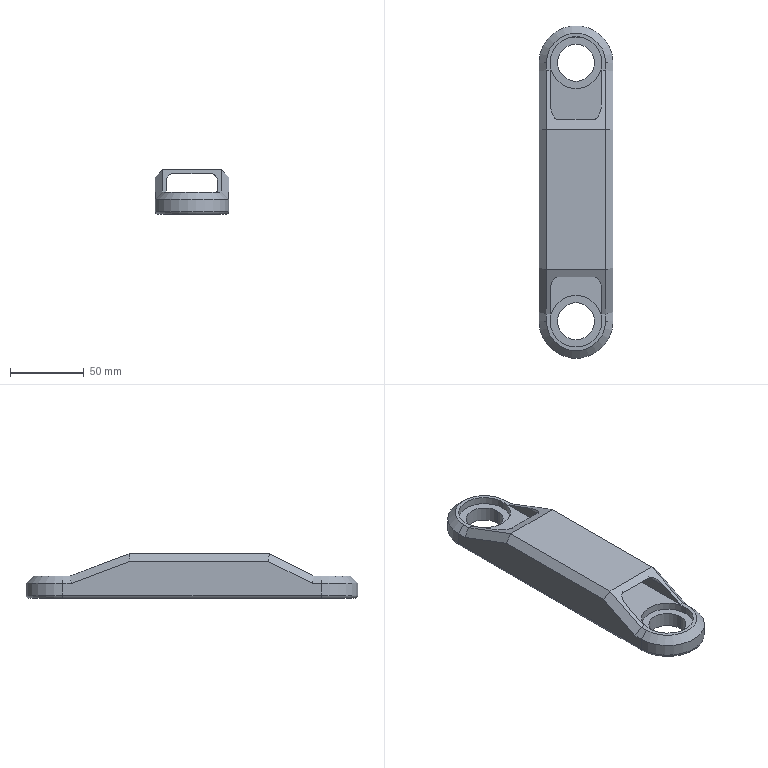Part | SolidWorks | features Cut 4, Fillet 2, Chamfer 1, Extrusion 1 | 1 solid | 40 faces | box 50 x 225 x 30 mm | volume 173740 mm3 | plane 22 | cylinder 14 | cone 2 | torus 2 | commonest cylinder face diameters 25 x4 35 x4 4 x2 10 x2 50 x2
STEP:
#1=CARTESIAN_POINT('',(-82.5,-150.,10.));
#2=VERTEX_POINT('',#1);
#3=CARTESIAN_POINT('',(-57.5,-150.,10.));
#4=VERTEX_POINT('',#3);
#5=CARTESIAN_POINT('',(-70.,-150.,10.));
#6=DIRECTION('',(0.,0.,1.));
#7=DIRECTION('',(1.,0.,0.));
#8=AXIS2_PLACEMENT_3D('',#5,#6,#7);
#9=CIRCLE('',#8,12.5);
#10=EDGE_CURVE('',#2,#4,#9,.T.);
#11=ORIENTED_EDGE('',*,*,#10,.T.);
#12=CARTESIAN_POINT('',(-57.5,-150.,0.));
#13=VERTEX_POINT('',#12);
#14=CARTESIAN_POINT('',(-57.5,-150.,30.));
#15=DIRECTION('',(0.,0.,-1.));
#16=VECTOR('',#15,1000.);
#17=LINE('',#14,#16);
#18=EDGE_CURVE('',#4,#13,#17,.T.);
#19=ORIENTED_EDGE('',*,*,#18,.T.);
#20=CARTESIAN_POINT('',(-82.5,-150.,0.));
#21=VERTEX_POINT('',#20);
#22=CARTESIAN_POINT('',(-70.,-150.,0.));
#23=DIRECTION('',(0.,0.,1.));
#24=DIRECTION('',(1.,0.,0.));
#25=AXIS2_PLACEMENT_3D('',#22,#23,#24);
#26=CIRCLE('',#25,12.5);
#27=EDGE_CURVE('',#21,#13,#26,.T.);
#28=ORIENTED_EDGE('',*,*,#27,.F.);
#29=CARTESIAN_POINT('',(-82.5,-150.,30.));
#30=DIRECTION('',(0.,0.,-1.));
#31=VECTOR('',#30,1000.);
#32=LINE('',#29,#31);
#33=EDGE_CURVE('',#2,#21,#32,.T.);
#34=ORIENTED_EDGE('',*,*,#33,.F.);
#35=EDGE_LOOP('',(#11,#19,#28,#34));
#36=FACE_OUTER_BOUND('',#35,.T.);
#37=CARTESIAN_POINT('',(-70.,-150.,30.));
#38=DIRECTION('',(0.,0.,-1.));
#39=DIRECTION('',(-1.,0.,0.));
#40=AXIS2_PLACEMENT_3D('',#37,#38,#39);
#41=CYLINDRICAL_SURFACE('',#40,12.5);
#42=ADVANCED_FACE('',(#36),#41,.F.);
#43=CARTESIAN_POINT('',(-82.5,25.,10.));
#44=VERTEX_POINT('',#43);
#45=CARTESIAN_POINT('',(-57.5,25.,10.));
#46=VERTEX_POINT('',#45);
#47=CARTESIAN_POINT('',(-70.,25.,10.));
#48=DIRECTION('',(0.,0.,1.));
#49=DIRECTION('',(1.,0.,0.));
#50=AXIS2_PLACEMENT_3D('',#47,#48,#49);
#51=CIRCLE('',#50,12.5);
#52=EDGE_CURVE('',#44,#46,#51,.T.);
#53=ORIENTED_EDGE('',*,*,#52,.T.);
#54=CARTESIAN_POINT('',(-57.5,25.,0.));
#55=VERTEX_POINT('',#54);
#56=CARTESIAN_POINT('',(-57.5,25.,30.));
#57=DIRECTION('',(0.,0.,-1.));
#58=VECTOR('',#57,1000.);
#59=LINE('',#56,#58);
#60=EDGE_CURVE('',#46,#55,#59,.T.);
#61=ORIENTED_EDGE('',*,*,#60,.T.);
#62=CARTESIAN_POINT('',(-82.5,25.,0.));
#63=VERTEX_POINT('',#62);
#64=CARTESIAN_POINT('',(-70.,25.,0.));
#65=DIRECTION('',(0.,0.,1.));
#66=DIRECTION('',(1.,0.,0.));
#67=AXIS2_PLACEMENT_3D('',#64,#65,#66);
#68=CIRCLE('',#67,12.5);
#69=EDGE_CURVE('',#63,#55,#68,.T.);
#70=ORIENTED_EDGE('',*,*,#69,.F.);
#71=CARTESIAN_POINT('',(-82.5,25.,30.));
#72=DIRECTION('',(0.,0.,-1.));
#73=VECTOR('',#72,1000.);
#74=LINE('',#71,#73);
#75=EDGE_CURVE('',#44,#63,#74,.T.);
#76=ORIENTED_EDGE('',*,*,#75,.F.);
#77=EDGE_LOOP('',(#53,#61,#70,#76));
#78=FACE_OUTER_BOUND('',#77,.T.);
#79=CARTESIAN_POINT('',(-70.,25.,30.));
#80=DIRECTION('',(0.,0.,-1.));
#81=DIRECTION('',(-1.,0.,0.));
#82=AXIS2_PLACEMENT_3D('',#79,#80,#81);
#83=CYLINDRICAL_SURFACE('',#82,12.5);
#84=ADVANCED_FACE('',(#78),#83,.F.);
#85=CARTESIAN_POINT('',(-87.5,25.,10.));
#86=VERTEX_POINT('',#85);
#87=CARTESIAN_POINT('',(-52.5,25.,10.));
#88=VERTEX_POINT('',#87);
#89=CARTESIAN_POINT('',(-70.,25.,10.));
#90=DIRECTION('',(0.,0.,1.));
#91=DIRECTION('',(1.,0.,0.));
#92=AXIS2_PLACEMENT_3D('',#89,#90,#91);
#93=CIRCLE('',#92,17.5);
#94=EDGE_CURVE('',#86,#88,#93,.T.);
#95=ORIENTED_EDGE('',*,*,#94,.F.);
#96=CARTESIAN_POINT('',(-87.5,25.,15.));
#97=VERTEX_POINT('',#96);
#98=CARTESIAN_POINT('',(-87.5,25.,10.));
#99=DIRECTION('',(0.,0.,1.));
#100=VECTOR('',#99,1000.);
#101=LINE('',#98,#100);
#102=EDGE_CURVE('',#86,#97,#101,.T.);
#103=ORIENTED_EDGE('',*,*,#102,.T.);
#104=CARTESIAN_POINT('',(-52.5,25.,15.));
#105=VERTEX_POINT('',#104);
#106=CARTESIAN_POINT('',(-70.,25.,15.));
#107=DIRECTION('',(0.,0.,-1.));
#108=DIRECTION('',(0.,1.,0.));
#109=AXIS2_PLACEMENT_3D('',#106,#107,#108);
#110=CIRCLE('',#109,17.5);
#111=EDGE_CURVE('',#105,#97,#110,.T.);
#112=ORIENTED_EDGE('',*,*,#111,.F.);
#113=CARTESIAN_POINT('',(-52.5,25.,10.));
#114=DIRECTION('',(0.,0.,1.));
#115=VECTOR('',#114,1000.);
#116=LINE('',#113,#115);
#117=EDGE_CURVE('',#88,#105,#116,.T.);
#118=ORIENTED_EDGE('',*,*,#117,.F.);
#119=EDGE_LOOP('',(#95,#103,#112,#118));
#120=FACE_OUTER_BOUND('',#119,.T.);
#121=CARTESIAN_POINT('',(-70.,25.,10.));
#122=DIRECTION('',(0.,0.,1.));
#123=DIRECTION('',(1.,0.,0.));
#124=AXIS2_PLACEMENT_3D('',#121,#122,#123);
#125=CYLINDRICAL_SURFACE('',#124,17.5);
#126=ADVANCED_FACE('',(#120),#125,.F.);
#127=CARTESIAN_POINT('',(-87.5,-150.,10.));
#128=VERTEX_POINT('',#127);
#129=CARTESIAN_POINT('',(-52.5,-150.,10.));
#130=VERTEX_POINT('',#129);
#131=CARTESIAN_POINT('',(-70.,-150.,10.));
#132=DIRECTION('',(0.,0.,1.));
#133=DIRECTION('',(1.,0.,0.));
#134=AXIS2_PLACEMENT_3D('',#131,#132,#133);
#135=CIRCLE('',#134,17.5);
#136=EDGE_CURVE('',#128,#130,#135,.T.);
#137=ORIENTED_EDGE('',*,*,#136,.F.);
#138=CARTESIAN_POINT('',(-87.5,-150.,15.));
#139=VERTEX_POINT('',#138);
#140=CARTESIAN_POINT('',(-87.5,-150.,10.));
#141=DIRECTION('',(0.,0.,1.));
#142=VECTOR('',#141,1000.);
#143=LINE('',#140,#142);
#144=EDGE_CURVE('',#128,#139,#143,.T.);
#145=ORIENTED_EDGE('',*,*,#144,.T.);
#146=CARTESIAN_POINT('',(-52.5,-150.,15.));
#147=VERTEX_POINT('',#146);
#148=CARTESIAN_POINT('',(-70.,-150.,15.));
#149=DIRECTION('',(0.,0.,-1.));
#150=DIRECTION('',(0.,1.,0.));
#151=AXIS2_PLACEMENT_3D('',#148,#149,#150);
#152=CIRCLE('',#151,17.5);
#153=EDGE_CURVE('',#147,#139,#152,.T.);
#154=ORIENTED_EDGE('',*,*,#153,.F.);
#155=CARTESIAN_POINT('',(-52.5,-150.,10.));
#156=DIRECTION('',(0.,0.,1.));
#157=VECTOR('',#156,1000.);
#158=LINE('',#155,#157);
#159=EDGE_CURVE('',#130,#147,#158,.T.);
#160=ORIENTED_EDGE('',*,*,#159,.F.);
#161=EDGE_LOOP('',(#137,#145,#154,#160));
#162=FACE_OUTER_BOUND('',#161,.T.);
#163=CARTESIAN_POINT('',(-70.,-150.,10.));
#164=DIRECTION('',(0.,0.,1.));
#165=DIRECTION('',(1.,0.,0.));
#166=AXIS2_PLACEMENT_3D('',#163,#164,#165);
#167=CYLINDRICAL_SURFACE('',#166,17.5);
#168=ADVANCED_FACE('',(#162),#167,.F.);
#169=CARTESIAN_POINT('',(-95.,25.,10.));
#170=VERTEX_POINT('',#169);
#171=CARTESIAN_POINT('',(-95.,25.,2.));
#172=VERTEX_POINT('',#171);
#173=CARTESIAN_POINT('',(-95.,25.,30.));
#174=DIRECTION('',(0.,0.,-1.));
#175=VECTOR('',#174,1000.);
#176=LINE('',#173,#175);
#177=EDGE_CURVE('',#170,#172,#176,.T.);
#178=ORIENTED_EDGE('',*,*,#177,.T.);
#179=CARTESIAN_POINT('',(-95.,-150.,2.));
#180=VERTEX_POINT('',#179);
#181=CARTESIAN_POINT('',(-95.,0.,2.));
#182=DIRECTION('',(0.,-1.,0.));
#183=VECTOR('',#182,1000.);
#184=LINE('',#181,#183);
#185=EDGE_CURVE('',#172,#180,#184,.T.);
#186=ORIENTED_EDGE('',*,*,#185,.T.);
#187=CARTESIAN_POINT('',(-95.,-150.,10.));
#188=VERTEX_POINT('',#187);
#189=CARTESIAN_POINT('',(-95.,-150.,30.));
#190=DIRECTION('',(0.,0.,-1.));
#191=VECTOR('',#190,1000.);
#192=LINE('',#189,#191);
#193=EDGE_CURVE('',#188,#180,#192,.T.);
#194=ORIENTED_EDGE('',*,*,#193,.F.);
#195=CARTESIAN_POINT('',(-95.,-143.82,10.));
#196=VERTEX_POINT('',#195);
#197=CARTESIAN_POINT('',(-95.,0.,10.));
#198=DIRECTION('',(0.,1.,0.));
#199=VECTOR('',#198,1000.);
#200=LINE('',#197,#199);
#201=EDGE_CURVE('',#188,#196,#200,.T.);
#202=ORIENTED_EDGE('',*,*,#201,.T.);
#203=CARTESIAN_POINT('',(-95.,-113.82,25.));
#204=VERTEX_POINT('',#203);
#205=CARTESIAN_POINT('',(-95.,-20.764,71.528));
#206=DIRECTION('',(0.,0.8944,0.4472));
#207=VECTOR('',#206,1000.);
#208=LINE('',#205,#207);
#209=EDGE_CURVE('',#196,#204,#208,.T.);
#210=ORIENTED_EDGE('',*,*,#209,.T.);
#211=CARTESIAN_POINT('',(-95.,-20.907,25.));
#212=VERTEX_POINT('',#211);
#213=CARTESIAN_POINT('',(-95.,-20.,25.));
#214=DIRECTION('',(0.,1.,0.));
#215=VECTOR('',#214,1000.);
#216=LINE('',#213,#215);
#217=EDGE_CURVE('',#204,#212,#216,.T.);
#218=ORIENTED_EDGE('',*,*,#217,.T.);
#219=CARTESIAN_POINT('',(-95.,19.093,10.));
#220=VERTEX_POINT('',#219);
#221=CARTESIAN_POINT('',(-95.,-4.221,18.743));
#222=DIRECTION('',(0.,0.9363,-0.3511));
#223=VECTOR('',#222,1000.);
#224=LINE('',#221,#223);
#225=EDGE_CURVE('',#212,#220,#224,.T.);
#226=ORIENTED_EDGE('',*,*,#225,.T.);
#227=CARTESIAN_POINT('',(-95.,0.,10.));
#228=DIRECTION('',(0.,1.,0.));
#229=VECTOR('',#228,1000.);
#230=LINE('',#227,#229);
#231=EDGE_CURVE('',#220,#170,#230,.T.);
#232=ORIENTED_EDGE('',*,*,#231,.T.);
#233=EDGE_LOOP('',(#178,#186,#194,#202,#210,#218,#226,#232));
#234=FACE_OUTER_BOUND('',#233,.T.);
#235=CARTESIAN_POINT('',(-95.,0.,30.));
#236=DIRECTION('',(1.,0.,0.));
#237=DIRECTION('',(0.,1.,0.));
#238=AXIS2_PLACEMENT_3D('',#235,#236,#237);
#239=PLANE('',#238);
#240=ADVANCED_FACE('',(#234),#239,.F.);
#241=ORIENTED_EDGE('',*,*,#193,.T.);
#242=CARTESIAN_POINT('',(-45.,-150.,2.));
#243=VERTEX_POINT('',#242);
#244=CARTESIAN_POINT('',(-70.,-150.,2.));
#245=DIRECTION('',(0.,0.,1.));
#246=DIRECTION('',(1.,0.,0.));
#247=AXIS2_PLACEMENT_3D('',#244,#245,#246);
#248=CIRCLE('',#247,25.);
#249=EDGE_CURVE('',#180,#243,#248,.T.);
#250=ORIENTED_EDGE('',*,*,#249,.T.);
#251=CARTESIAN_POINT('',(-45.,-150.,10.));
#252=VERTEX_POINT('',#251);
#253=CARTESIAN_POINT('',(-45.,-150.,30.));
#254=DIRECTION('',(0.,0.,-1.));
#255=VECTOR('',#254,1000.);
#256=LINE('',#253,#255);
#257=EDGE_CURVE('',#252,#243,#256,.T.);
#258=ORIENTED_EDGE('',*,*,#257,.F.);
#259=CARTESIAN_POINT('',(-70.,-150.,10.));
#260=DIRECTION('',(0.,0.,-1.));
#261=DIRECTION('',(-1.,0.,0.));
#262=AXIS2_PLACEMENT_3D('',#259,#260,#261);
#263=CIRCLE('',#262,25.);
#264=EDGE_CURVE('',#252,#188,#263,.T.);
#265=ORIENTED_EDGE('',*,*,#264,.T.);
#266=EDGE_LOOP('',(#241,#250,#258,#265));
#267=FACE_OUTER_BOUND('',#266,.T.);
#268=CARTESIAN_POINT('',(-70.,-150.,30.));
#269=DIRECTION('',(0.,0.,-1.));
#270=DIRECTION('',(-1.,0.,0.));
#271=AXIS2_PLACEMENT_3D('',#268,#269,#270);
#272=CYLINDRICAL_SURFACE('',#271,25.);
#273=ADVANCED_FACE('',(#267),#272,.T.);
#274=ORIENTED_EDGE('',*,*,#257,.T.);
#275=CARTESIAN_POINT('',(-45.,25.,2.));
#276=VERTEX_POINT('',#275);
#277=CARTESIAN_POINT('',(-45.,25.,2.));
#278=DIRECTION('',(0.,1.,0.));
#279=VECTOR('',#278,1000.);
#280=LINE('',#277,#279);
#281=EDGE_CURVE('',#243,#276,#280,.T.);
#282=ORIENTED_EDGE('',*,*,#281,.T.);
#283=CARTESIAN_POINT('',(-45.,25.,10.));
#284=VERTEX_POINT('',#283);
#285=CARTESIAN_POINT('',(-45.,25.,30.));
#286=DIRECTION('',(0.,0.,-1.));
#287=VECTOR('',#286,1000.);
#288=LINE('',#285,#287);
#289=EDGE_CURVE('',#284,#276,#288,.T.);
#290=ORIENTED_EDGE('',*,*,#289,.F.);
#291=CARTESIAN_POINT('',(-45.,19.093,10.));
#292=VERTEX_POINT('',#291);
#293=CARTESIAN_POINT('',(-45.,20.,10.));
#294=DIRECTION('',(0.,-1.,0.));
#295=VECTOR('',#294,1000.);
#296=LINE('',#293,#295);
#297=EDGE_CURVE('',#284,#292,#296,.T.);
#298=ORIENTED_EDGE('',*,*,#297,.T.);
#299=CARTESIAN_POINT('',(-45.,-20.907,25.));
#300=VERTEX_POINT('',#299);
#301=CARTESIAN_POINT('',(-45.,-21.756,25.318));
#302=DIRECTION('',(0.,-0.9363,0.3511));
#303=VECTOR('',#302,1000.);
#304=LINE('',#301,#303);
#305=EDGE_CURVE('',#292,#300,#304,.T.);
#306=ORIENTED_EDGE('',*,*,#305,.T.);
#307=CARTESIAN_POINT('',(-45.,-113.82,25.));
#308=VERTEX_POINT('',#307);
#309=CARTESIAN_POINT('',(-45.,0.,25.));
#310=DIRECTION('',(0.,-1.,0.));
#311=VECTOR('',#310,1000.);
#312=LINE('',#309,#311);
#313=EDGE_CURVE('',#300,#308,#312,.T.);
#314=ORIENTED_EDGE('',*,*,#313,.T.);
#315=CARTESIAN_POINT('',(-45.,-143.82,10.));
#316=VERTEX_POINT('',#315);
#317=CARTESIAN_POINT('',(-45.,-142.764,10.528));
#318=DIRECTION('',(0.,-0.8944,-0.4472));
#319=VECTOR('',#318,1000.);
#320=LINE('',#317,#319);
#321=EDGE_CURVE('',#308,#316,#320,.T.);
#322=ORIENTED_EDGE('',*,*,#321,.T.);
#323=CARTESIAN_POINT('',(-45.,-150.,10.));
#324=DIRECTION('',(0.,-1.,0.));
#325=VECTOR('',#324,1000.);
#326=LINE('',#323,#325);
#327=EDGE_CURVE('',#316,#252,#326,.T.);
#328=ORIENTED_EDGE('',*,*,#327,.T.);
#329=EDGE_LOOP('',(#274,#282,#290,#298,#306,#314,#322,#328));
#330=FACE_OUTER_BOUND('',#329,.T.);
#331=CARTESIAN_POINT('',(-45.,0.,30.));
#332=DIRECTION('',(1.,0.,0.));
#333=DIRECTION('',(0.,1.,0.));
#334=AXIS2_PLACEMENT_3D('',#331,#332,#333);
#335=PLANE('',#334);
#336=ADVANCED_FACE('',(#330),#335,.T.);
#337=ORIENTED_EDGE('',*,*,#289,.T.);
#338=CARTESIAN_POINT('',(-70.,25.,2.));
#339=DIRECTION('',(0.,0.,1.));
#340=DIRECTION('',(1.,0.,0.));
#341=AXIS2_PLACEMENT_3D('',#338,#339,#340);
#342=CIRCLE('',#341,25.);
#343=EDGE_CURVE('',#276,#172,#342,.T.);
#344=ORIENTED_EDGE('',*,*,#343,.T.);
#345=ORIENTED_EDGE('',*,*,#177,.F.);
#346=CARTESIAN_POINT('',(-70.,25.,10.));
#347=DIRECTION('',(0.,0.,-1.));
#348=DIRECTION('',(-1.,0.,0.));
#349=AXIS2_PLACEMENT_3D('',#346,#347,#348);
#350=CIRCLE('',#349,25.);
#351=EDGE_CURVE('',#170,#284,#350,.T.);
#352=ORIENTED_EDGE('',*,*,#351,.T.);
#353=EDGE_LOOP('',(#337,#344,#345,#352));
#354=FACE_OUTER_BOUND('',#353,.T.);
#355=CARTESIAN_POINT('',(-70.,25.,30.));
#356=DIRECTION('',(0.,0.,-1.));
#357=DIRECTION('',(-1.,0.,0.));
#358=AXIS2_PLACEMENT_3D('',#355,#356,#357);
#359=CYLINDRICAL_SURFACE('',#358,25.);
#360=ADVANCED_FACE('',(#354),#359,.T.);
#361=CARTESIAN_POINT('',(-90.,-115.,30.));
#362=VERTEX_POINT('',#361);
#363=CARTESIAN_POINT('',(-50.,-115.,30.));
#364=VERTEX_POINT('',#363);
#365=CARTESIAN_POINT('',(-95.,-115.,30.));
#366=DIRECTION('',(1.,0.,0.));
#367=VECTOR('',#366,1000.);
#368=LINE('',#365,#367);
#369=EDGE_CURVE('',#362,#364,#368,.T.);
#370=ORIENTED_EDGE('',*,*,#369,.T.);
#371=CARTESIAN_POINT('',(-50.,-20.,30.));
#372=VERTEX_POINT('',#371);
#373=CARTESIAN_POINT('',(-50.,0.,30.));
#374=DIRECTION('',(0.,1.,0.));
#375=VECTOR('',#374,1000.);
#376=LINE('',#373,#375);
#377=EDGE_CURVE('',#364,#372,#376,.T.);
#378=ORIENTED_EDGE('',*,*,#377,.T.);
#379=CARTESIAN_POINT('',(-90.,-20.,30.));
#380=VERTEX_POINT('',#379);
#381=CARTESIAN_POINT('',(-95.,-20.,30.));
#382=DIRECTION('',(1.,0.,0.));
#383=VECTOR('',#382,1000.);
#384=LINE('',#381,#383);
#385=EDGE_CURVE('',#380,#372,#384,.T.);
#386=ORIENTED_EDGE('',*,*,#385,.F.);
#387=CARTESIAN_POINT('',(-90.,-115.,30.));
#388=DIRECTION('',(0.,-1.,0.));
#389=VECTOR('',#388,1000.);
#390=LINE('',#387,#389);
#391=EDGE_CURVE('',#380,#362,#390,.T.);
#392=ORIENTED_EDGE('',*,*,#391,.T.);
#393=EDGE_LOOP('',(#370,#378,#386,#392));
#394=FACE_OUTER_BOUND('',#393,.T.);
#395=CARTESIAN_POINT('',(0.,0.,30.));
#396=DIRECTION('',(0.,0.,1.));
#397=DIRECTION('',(1.,0.,0.));
#398=AXIS2_PLACEMENT_3D('',#395,#396,#397);
#399=PLANE('',#398);
#400=ADVANCED_FACE('',(#394),#399,.T.);
#401=CARTESIAN_POINT('',(-93.,-150.,0.));
#402=VERTEX_POINT('',#401);
#403=CARTESIAN_POINT('',(-93.,25.,0.));
#404=VERTEX_POINT('',#403);
#405=CARTESIAN_POINT('',(-93.,0.,0.));
#406=DIRECTION('',(0.,1.,0.));
#407=VECTOR('',#406,1000.);
#408=LINE('',#405,#407);
#409=EDGE_CURVE('',#402,#404,#408,.T.);
#410=ORIENTED_EDGE('',*,*,#409,.T.);
#411=CARTESIAN_POINT('',(-47.,25.,0.));
#412=VERTEX_POINT('',#411);
#413=CARTESIAN_POINT('',(-70.,25.,0.));
#414=DIRECTION('',(0.,0.,-1.));
#415=DIRECTION('',(1.,0.,0.));
#416=AXIS2_PLACEMENT_3D('',#413,#414,#415);
#417=CIRCLE('',#416,23.);
#418=EDGE_CURVE('',#404,#412,#417,.T.);
#419=ORIENTED_EDGE('',*,*,#418,.T.);
#420=CARTESIAN_POINT('',(-47.,-150.,0.));
#421=VERTEX_POINT('',#420);
#422=CARTESIAN_POINT('',(-47.,-150.,0.));
#423=DIRECTION('',(0.,-1.,0.));
#424=VECTOR('',#423,1000.);
#425=LINE('',#422,#424);
#426=EDGE_CURVE('',#412,#421,#425,.T.);
#427=ORIENTED_EDGE('',*,*,#426,.T.);
#428=CARTESIAN_POINT('',(-70.,-150.,0.));
#429=DIRECTION('',(0.,0.,-1.));
#430=DIRECTION('',(1.,0.,0.));
#431=AXIS2_PLACEMENT_3D('',#428,#429,#430);
#432=CIRCLE('',#431,23.);
#433=EDGE_CURVE('',#421,#402,#432,.T.);
#434=ORIENTED_EDGE('',*,*,#433,.T.);
#435=EDGE_LOOP('',(#410,#419,#427,#434));
#436=FACE_OUTER_BOUND('',#435,.T.);
#437=ORIENTED_EDGE('',*,*,#69,.T.);
#438=CARTESIAN_POINT('',(-70.,25.,0.));
#439=DIRECTION('',(0.,0.,1.));
#440=DIRECTION('',(1.,0.,0.));
#441=AXIS2_PLACEMENT_3D('',#438,#439,#440);
#442=CIRCLE('',#441,12.5);
#443=EDGE_CURVE('',#55,#63,#442,.T.);
#444=ORIENTED_EDGE('',*,*,#443,.T.);
#445=EDGE_LOOP('',(#437,#444));
#446=FACE_BOUND('',#445,.T.);
#447=ORIENTED_EDGE('',*,*,#27,.T.);
#448=CARTESIAN_POINT('',(-70.,-150.,0.));
#449=DIRECTION('',(0.,0.,1.));
#450=DIRECTION('',(1.,0.,0.));
#451=AXIS2_PLACEMENT_3D('',#448,#449,#450);
#452=CIRCLE('',#451,12.5);
#453=EDGE_CURVE('',#13,#21,#452,.T.);
#454=ORIENTED_EDGE('',*,*,#453,.T.);
#455=EDGE_LOOP('',(#447,#454));
#456=FACE_BOUND('',#455,.T.);
#457=CARTESIAN_POINT('',(0.,0.,0.));
#458=DIRECTION('',(0.,0.,1.));
#459=DIRECTION('',(1.,0.,0.));
#460=AXIS2_PLACEMENT_3D('',#457,#458,#459);
#461=PLANE('',#460);
#462=ADVANCED_FACE('',(#436,#446,#456),#461,.F.);
#463=CARTESIAN_POINT('',(-52.5,20.,15.));
#464=VERTEX_POINT('',#463);
#465=CARTESIAN_POINT('',(-52.5,0.,22.5));
#466=VERTEX_POINT('',#465);
#467=CARTESIAN_POINT('',(-52.5,20.,15.));
#468=DIRECTION('',(0.,-0.9363,0.3511));
#469=VECTOR('',#468,1000.);
#470=LINE('',#467,#469);
#471=EDGE_CURVE('',#464,#466,#470,.T.);
#472=ORIENTED_EDGE('',*,*,#471,.T.);
#473=CARTESIAN_POINT('',(-57.5,-13.333,27.5));
#474=VERTEX_POINT('',#473);
#475=CARTESIAN_POINT('',(-52.5,0.,22.5));
#476=CARTESIAN_POINT('',(-52.5,-7.81,25.429));
#477=CARTESIAN_POINT('',(-54.571,-13.333,27.5));
#478=CARTESIAN_POINT('',(-57.5,-13.333,27.5));
#479=(BOUNDED_CURVE()B_SPLINE_CURVE(3,(#475,#476,#477,#478),.UNSPECIFIED.,.F.,.F.)B_SPLINE_CURVE_WITH_KNOTS((4,4),(4.712,6.283),.UNSPECIFIED.)CURVE()GEOMETRIC_REPRESENTATION_ITEM()RATIONAL_B_SPLINE_CURVE((1.,0.8047,0.8047,1.))REPRESENTATION_ITEM(''));
#480=EDGE_CURVE('',#466,#474,#479,.T.);
#481=ORIENTED_EDGE('',*,*,#480,.T.);
#482=CARTESIAN_POINT('',(-82.5,-13.333,27.5));
#483=VERTEX_POINT('',#482);
#484=CARTESIAN_POINT('',(-95.,-13.333,27.5));
#485=DIRECTION('',(-1.,0.,0.));
#486=VECTOR('',#485,1000.);
#487=LINE('',#484,#486);
#488=EDGE_CURVE('',#474,#483,#487,.T.);
#489=ORIENTED_EDGE('',*,*,#488,.T.);
#490=CARTESIAN_POINT('',(-87.5,0.,22.5));
#491=VERTEX_POINT('',#490);
#492=CARTESIAN_POINT('',(-82.5,-13.333,27.5));
#493=CARTESIAN_POINT('',(-85.429,-13.333,27.5));
#494=CARTESIAN_POINT('',(-87.5,-7.81,25.429));
#495=CARTESIAN_POINT('',(-87.5,0.,22.5));
#496=(BOUNDED_CURVE()B_SPLINE_CURVE(3,(#492,#493,#494,#495),.UNSPECIFIED.,.F.,.T.)B_SPLINE_CURVE_WITH_KNOTS((4,4),(0.,1.571),.UNSPECIFIED.)CURVE()GEOMETRIC_REPRESENTATION_ITEM()RATIONAL_B_SPLINE_CURVE((1.,0.8047,0.8047,1.))REPRESENTATION_ITEM(''));
#497=EDGE_CURVE('',#483,#491,#496,.T.);
#498=ORIENTED_EDGE('',*,*,#497,.T.);
#499=CARTESIAN_POINT('',(-87.5,20.,15.));
#500=VERTEX_POINT('',#499);
#501=CARTESIAN_POINT('',(-87.5,20.,15.));
#502=DIRECTION('',(0.,0.9363,-0.3511));
#503=VECTOR('',#502,1000.);
#504=LINE('',#501,#503);
#505=EDGE_CURVE('',#491,#500,#504,.T.);
#506=ORIENTED_EDGE('',*,*,#505,.T.);
#507=CARTESIAN_POINT('',(-90.,20.,15.));
#508=VERTEX_POINT('',#507);
#509=CARTESIAN_POINT('',(-95.,20.,15.));
#510=DIRECTION('',(1.,0.,0.));
#511=VECTOR('',#510,1000.);
#512=LINE('',#509,#511);
#513=EDGE_CURVE('',#508,#500,#512,.T.);
#514=ORIENTED_EDGE('',*,*,#513,.F.);
#515=CARTESIAN_POINT('',(-90.,20.,15.));
#516=DIRECTION('',(0.,-0.9363,0.3511));
#517=VECTOR('',#516,1000.);
#518=LINE('',#515,#517);
#519=EDGE_CURVE('',#508,#380,#518,.T.);
#520=ORIENTED_EDGE('',*,*,#519,.T.);
#521=ORIENTED_EDGE('',*,*,#385,.T.);
#522=CARTESIAN_POINT('',(-50.,20.,15.));
#523=VERTEX_POINT('',#522);
#524=CARTESIAN_POINT('',(-50.,20.,15.));
#525=DIRECTION('',(0.,0.9363,-0.3511));
#526=VECTOR('',#525,1000.);
#527=LINE('',#524,#526);
#528=EDGE_CURVE('',#372,#523,#527,.T.);
#529=ORIENTED_EDGE('',*,*,#528,.T.);
#530=CARTESIAN_POINT('',(-95.,20.,15.));
#531=DIRECTION('',(1.,0.,0.));
#532=VECTOR('',#531,1000.);
#533=LINE('',#530,#532);
#534=EDGE_CURVE('',#464,#523,#533,.T.);
#535=ORIENTED_EDGE('',*,*,#534,.F.);
#536=EDGE_LOOP('',(#472,#481,#489,#498,#506,#514,#520,#521,#529,#535));
#537=FACE_OUTER_BOUND('',#536,.T.);
#538=CARTESIAN_POINT('',(-95.,20.,15.));
#539=DIRECTION('',(0.,-0.3511,-0.9363));
#540=DIRECTION('',(0.,0.9363,-0.3511));
#541=AXIS2_PLACEMENT_3D('',#538,#539,#540);
#542=PLANE('',#541);
#543=ADVANCED_FACE('',(#537),#542,.F.);
#544=ORIENTED_EDGE('',*,*,#111,.T.);
#545=CARTESIAN_POINT('',(-70.,25.,15.));
#546=DIRECTION('',(0.,0.,-1.));
#547=DIRECTION('',(0.,1.,0.));
#548=AXIS2_PLACEMENT_3D('',#545,#546,#547);
#549=CIRCLE('',#548,17.5);
#550=EDGE_CURVE('',#97,#105,#549,.T.);
#551=ORIENTED_EDGE('',*,*,#550,.T.);
#552=EDGE_LOOP('',(#544,#551));
#553=FACE_BOUND('',#552,.T.);
#554=ORIENTED_EDGE('',*,*,#153,.T.);
#555=CARTESIAN_POINT('',(-70.,-150.,15.));
#556=DIRECTION('',(0.,0.,-1.));
#557=DIRECTION('',(0.,1.,0.));
#558=AXIS2_PLACEMENT_3D('',#555,#556,#557);
#559=CIRCLE('',#558,17.5);
#560=EDGE_CURVE('',#139,#147,#559,.T.);
#561=ORIENTED_EDGE('',*,*,#560,.T.);
#562=EDGE_LOOP('',(#554,#561));
#563=FACE_BOUND('',#562,.T.);
#564=CARTESIAN_POINT('',(-52.5,-145.,15.));
#565=VERTEX_POINT('',#564);
#566=CARTESIAN_POINT('',(-50.,-145.,15.));
#567=VERTEX_POINT('',#566);
#568=CARTESIAN_POINT('',(-95.,-145.,15.));
#569=DIRECTION('',(1.,0.,0.));
#570=VECTOR('',#569,1000.);
#571=LINE('',#568,#570);
#572=EDGE_CURVE('',#565,#567,#571,.T.);
#573=ORIENTED_EDGE('',*,*,#572,.F.);
#574=CARTESIAN_POINT('',(-52.5,-175.,15.));
#575=DIRECTION('',(0.,1.,0.));
#576=VECTOR('',#575,1000.);
#577=LINE('',#574,#576);
#578=EDGE_CURVE('',#565,#464,#577,.T.);
#579=ORIENTED_EDGE('',*,*,#578,.T.);
#580=ORIENTED_EDGE('',*,*,#534,.T.);
#581=CARTESIAN_POINT('',(-50.,25.,15.));
#582=VERTEX_POINT('',#581);
#583=CARTESIAN_POINT('',(-50.,25.,15.));
#584=DIRECTION('',(0.,1.,0.));
#585=VECTOR('',#584,1000.);
#586=LINE('',#583,#585);
#587=EDGE_CURVE('',#523,#582,#586,.T.);
#588=ORIENTED_EDGE('',*,*,#587,.T.);
#589=CARTESIAN_POINT('',(-90.,25.,15.));
#590=VERTEX_POINT('',#589);
#591=CARTESIAN_POINT('',(-70.,25.,15.));
#592=DIRECTION('',(0.,0.,1.));
#593=DIRECTION('',(0.,1.,0.));
#594=AXIS2_PLACEMENT_3D('',#591,#592,#593);
#595=CIRCLE('',#594,20.);
#596=EDGE_CURVE('',#582,#590,#595,.T.);
#597=ORIENTED_EDGE('',*,*,#596,.T.);
#598=CARTESIAN_POINT('',(-90.,20.,15.));
#599=DIRECTION('',(0.,-1.,0.));
#600=VECTOR('',#599,1000.);
#601=LINE('',#598,#600);
#602=EDGE_CURVE('',#590,#508,#601,.T.);
#603=ORIENTED_EDGE('',*,*,#602,.T.);
#604=ORIENTED_EDGE('',*,*,#513,.T.);
#605=CARTESIAN_POINT('',(-87.5,-145.,15.));
#606=VERTEX_POINT('',#605);
#607=CARTESIAN_POINT('',(-87.5,-175.,15.));
#608=DIRECTION('',(0.,1.,0.));
#609=VECTOR('',#608,1000.);
#610=LINE('',#607,#609);
#611=EDGE_CURVE('',#606,#500,#610,.T.);
#612=ORIENTED_EDGE('',*,*,#611,.F.);
#613=CARTESIAN_POINT('',(-90.,-145.,15.));
#614=VERTEX_POINT('',#613);
#615=CARTESIAN_POINT('',(-95.,-145.,15.));
#616=DIRECTION('',(1.,0.,0.));
#617=VECTOR('',#616,1000.);
#618=LINE('',#615,#617);
#619=EDGE_CURVE('',#614,#606,#618,.T.);
#620=ORIENTED_EDGE('',*,*,#619,.F.);
#621=CARTESIAN_POINT('',(-90.,-150.,15.));
#622=VERTEX_POINT('',#621);
#623=CARTESIAN_POINT('',(-90.,-145.,15.));
#624=DIRECTION('',(0.,-1.,0.));
#625=VECTOR('',#624,1000.);
#626=LINE('',#623,#625);
#627=EDGE_CURVE('',#614,#622,#626,.T.);
#628=ORIENTED_EDGE('',*,*,#627,.T.);
#629=CARTESIAN_POINT('',(-50.,-150.,15.));
#630=VERTEX_POINT('',#629);
#631=CARTESIAN_POINT('',(-70.,-150.,15.));
#632=DIRECTION('',(0.,0.,1.));
#633=DIRECTION('',(0.,1.,0.));
#634=AXIS2_PLACEMENT_3D('',#631,#632,#633);
#635=CIRCLE('',#634,20.);
#636=EDGE_CURVE('',#622,#630,#635,.T.);
#637=ORIENTED_EDGE('',*,*,#636,.T.);
#638=CARTESIAN_POINT('',(-50.,-145.,15.));
#639=DIRECTION('',(0.,1.,0.));
#640=VECTOR('',#639,1000.);
#641=LINE('',#638,#640);
#642=EDGE_CURVE('',#630,#567,#641,.T.);
#643=ORIENTED_EDGE('',*,*,#642,.T.);
#644=EDGE_LOOP('',(#573,#579,#580,#588,#597,#603,#604,#612,#620,#628,#637,#643));
#645=FACE_OUTER_BOUND('',#644,.T.);
#646=CARTESIAN_POINT('',(-95.,-145.,15.));
#647=DIRECTION('',(0.,0.,-1.));
#648=DIRECTION('',(0.,1.,0.));
#649=AXIS2_PLACEMENT_3D('',#646,#647,#648);
#650=PLANE('',#649);
#651=ADVANCED_FACE('',(#553,#563,#645),#650,.F.);
#652=ORIENTED_EDGE('',*,*,#619,.T.);
#653=CARTESIAN_POINT('',(-87.5,-130.,22.5));
#654=VERTEX_POINT('',#653);
#655=CARTESIAN_POINT('',(-87.5,-115.,30.));
#656=DIRECTION('',(0.,0.8944,0.4472));
#657=VECTOR('',#656,1000.);
#658=LINE('',#655,#657);
#659=EDGE_CURVE('',#606,#654,#658,.T.);
#660=ORIENTED_EDGE('',*,*,#659,.T.);
#661=CARTESIAN_POINT('',(-82.5,-120.,27.5));
#662=VERTEX_POINT('',#661);
#663=CARTESIAN_POINT('',(-87.5,-130.,22.5));
#664=CARTESIAN_POINT('',(-87.5,-124.142,25.429));
#665=CARTESIAN_POINT('',(-85.429,-120.,27.5));
#666=CARTESIAN_POINT('',(-82.5,-120.,27.5));
#667=(BOUNDED_CURVE()B_SPLINE_CURVE(3,(#663,#664,#665,#666),.UNSPECIFIED.,.F.,.F.)B_SPLINE_CURVE_WITH_KNOTS((4,4),(1.571,3.142),.UNSPECIFIED.)CURVE()GEOMETRIC_REPRESENTATION_ITEM()RATIONAL_B_SPLINE_CURVE((1.,0.8047,0.8047,1.))REPRESENTATION_ITEM(''));
#668=EDGE_CURVE('',#654,#662,#667,.T.);
#669=ORIENTED_EDGE('',*,*,#668,.T.);
#670=CARTESIAN_POINT('',(-57.5,-120.,27.5));
#671=VERTEX_POINT('',#670);
#672=CARTESIAN_POINT('',(-95.,-120.,27.5));
#673=DIRECTION('',(1.,0.,0.));
#674=VECTOR('',#673,1000.);
#675=LINE('',#672,#674);
#676=EDGE_CURVE('',#662,#671,#675,.T.);
#677=ORIENTED_EDGE('',*,*,#676,.T.);
#678=CARTESIAN_POINT('',(-52.5,-130.,22.5));
#679=VERTEX_POINT('',#678);
#680=CARTESIAN_POINT('',(-57.5,-120.,27.5));
#681=CARTESIAN_POINT('',(-54.571,-120.,27.5));
#682=CARTESIAN_POINT('',(-52.5,-124.142,25.429));
#683=CARTESIAN_POINT('',(-52.5,-130.,22.5));
#684=(BOUNDED_CURVE()B_SPLINE_CURVE(3,(#680,#681,#682,#683),.UNSPECIFIED.,.F.,.T.)B_SPLINE_CURVE_WITH_KNOTS((4,4),(3.142,4.712),.UNSPECIFIED.)CURVE()GEOMETRIC_REPRESENTATION_ITEM()RATIONAL_B_SPLINE_CURVE((1.,0.8047,0.8047,1.))REPRESENTATION_ITEM(''));
#685=EDGE_CURVE('',#671,#679,#684,.T.);
#686=ORIENTED_EDGE('',*,*,#685,.T.);
#687=CARTESIAN_POINT('',(-52.5,-115.,30.));
#688=DIRECTION('',(0.,-0.8944,-0.4472));
#689=VECTOR('',#688,1000.);
#690=LINE('',#687,#689);
#691=EDGE_CURVE('',#679,#565,#690,.T.);
#692=ORIENTED_EDGE('',*,*,#691,.T.);
#693=ORIENTED_EDGE('',*,*,#572,.T.);
#694=CARTESIAN_POINT('',(-50.,-115.,30.));
#695=DIRECTION('',(0.,0.8944,0.4472));
#696=VECTOR('',#695,1000.);
#697=LINE('',#694,#696);
#698=EDGE_CURVE('',#567,#364,#697,.T.);
#699=ORIENTED_EDGE('',*,*,#698,.T.);
#700=ORIENTED_EDGE('',*,*,#369,.F.);
#701=CARTESIAN_POINT('',(-90.,-115.,30.));
#702=DIRECTION('',(0.,-0.8944,-0.4472));
#703=VECTOR('',#702,1000.);
#704=LINE('',#701,#703);
#705=EDGE_CURVE('',#362,#614,#704,.T.);
#706=ORIENTED_EDGE('',*,*,#705,.T.);
#707=EDGE_LOOP('',(#652,#660,#669,#677,#686,#692,#693,#699,#700,#706));
#708=FACE_OUTER_BOUND('',#707,.T.);
#709=CARTESIAN_POINT('',(-95.,-115.,30.));
#710=DIRECTION('',(0.,0.4472,-0.8944));
#711=DIRECTION('',(0.,0.8944,0.4472));
#712=AXIS2_PLACEMENT_3D('',#709,#710,#711);
#713=PLANE('',#712);
#714=ADVANCED_FACE('',(#708),#713,.F.);
#715=CARTESIAN_POINT('',(-50.,25.,15.));
#716=DIRECTION('',(0.7071,0.,-0.7071));
#717=VECTOR('',#716,1000.);
#718=LINE('',#715,#717);
#719=EDGE_CURVE('',#582,#284,#718,.T.);
#720=ORIENTED_EDGE('',*,*,#719,.F.);
#721=ORIENTED_EDGE('',*,*,#587,.F.);
#722=CARTESIAN_POINT('',(-50.,20.,15.));
#723=DIRECTION('',(-0.7014,0.1272,0.7014));
#724=VECTOR('',#723,1000.);
#725=LINE('',#722,#724);
#726=EDGE_CURVE('',#292,#523,#725,.T.);
#727=ORIENTED_EDGE('',*,*,#726,.F.);
#728=ORIENTED_EDGE('',*,*,#297,.F.);
#729=EDGE_LOOP('',(#720,#721,#727,#728));
#730=FACE_OUTER_BOUND('',#729,.T.);
#731=CARTESIAN_POINT('',(-50.,20.,15.));
#732=DIRECTION('',(0.7071,0.,0.7071));
#733=DIRECTION('',(0.,-1.,0.));
#734=AXIS2_PLACEMENT_3D('',#731,#732,#733);
#735=PLANE('',#734);
#736=ADVANCED_FACE('',(#730),#735,.T.);
#737=ORIENTED_EDGE('',*,*,#726,.T.);
#738=ORIENTED_EDGE('',*,*,#528,.F.);
#739=CARTESIAN_POINT('',(-46.189,-20.691,26.189));
#740=DIRECTION('',(-0.7014,0.1272,0.7014));
#741=VECTOR('',#740,1000.);
#742=LINE('',#739,#741);
#743=EDGE_CURVE('',#300,#372,#742,.T.);
#744=ORIENTED_EDGE('',*,*,#743,.F.);
#745=ORIENTED_EDGE('',*,*,#305,.F.);
#746=EDGE_LOOP('',(#737,#738,#744,#745));
#747=FACE_OUTER_BOUND('',#746,.T.);
#748=CARTESIAN_POINT('',(-50.,20.,15.));
#749=DIRECTION('',(0.7071,0.2483,0.6621));
#750=DIRECTION('',(0.,-0.9363,0.3511));
#751=AXIS2_PLACEMENT_3D('',#748,#749,#750);
#752=PLANE('',#751);
#753=ADVANCED_FACE('',(#747),#752,.T.);
#754=ORIENTED_EDGE('',*,*,#719,.T.);
#755=ORIENTED_EDGE('',*,*,#351,.F.);
#756=CARTESIAN_POINT('',(-90.,25.,15.));
#757=DIRECTION('',(-0.7071,0.,-0.7071));
#758=VECTOR('',#757,1000.);
#759=LINE('',#756,#758);
#760=EDGE_CURVE('',#590,#170,#759,.T.);
#761=ORIENTED_EDGE('',*,*,#760,.F.);
#762=ORIENTED_EDGE('',*,*,#596,.F.);
#763=EDGE_LOOP('',(#754,#755,#761,#762));
#764=FACE_OUTER_BOUND('',#763,.T.);
#765=CARTESIAN_POINT('',(-70.,25.,10.));
#766=DIRECTION('',(0.,0.,-1.));
#767=DIRECTION('',(-1.,0.,0.));
#768=AXIS2_PLACEMENT_3D('',#765,#766,#767);
#769=CONICAL_SURFACE('',#768,25.,0.7854);
#770=ADVANCED_FACE('',(#764),#769,.T.);
#771=ORIENTED_EDGE('',*,*,#743,.T.);
#772=ORIENTED_EDGE('',*,*,#377,.F.);
#773=CARTESIAN_POINT('',(-31.93,-110.734,11.93));
#774=DIRECTION('',(-0.6975,-0.1646,0.6975));
#775=VECTOR('',#774,1000.);
#776=LINE('',#773,#775);
#777=EDGE_CURVE('',#308,#364,#776,.T.);
#778=ORIENTED_EDGE('',*,*,#777,.F.);
#779=ORIENTED_EDGE('',*,*,#313,.F.);
#780=EDGE_LOOP('',(#771,#772,#778,#779));
#781=FACE_OUTER_BOUND('',#780,.T.);
#782=CARTESIAN_POINT('',(-45.,0.,25.));
#783=DIRECTION('',(-0.7071,0.,-0.7071));
#784=DIRECTION('',(0.,-1.,0.));
#785=AXIS2_PLACEMENT_3D('',#782,#783,#784);
#786=PLANE('',#785);
#787=ADVANCED_FACE('',(#781),#786,.F.);
#788=ORIENTED_EDGE('',*,*,#760,.T.);
#789=ORIENTED_EDGE('',*,*,#231,.F.);
#790=CARTESIAN_POINT('',(-96.703,18.784,8.297));
#791=DIRECTION('',(-0.7014,-0.1272,-0.7014));
#792=VECTOR('',#791,1000.);
#793=LINE('',#790,#792);
#794=EDGE_CURVE('',#508,#220,#793,.T.);
#795=ORIENTED_EDGE('',*,*,#794,.F.);
#796=ORIENTED_EDGE('',*,*,#602,.F.);
#797=EDGE_LOOP('',(#788,#789,#795,#796));
#798=FACE_OUTER_BOUND('',#797,.T.);
#799=CARTESIAN_POINT('',(-95.,0.,10.));
#800=DIRECTION('',(0.7071,0.,-0.7071));
#801=DIRECTION('',(0.,1.,0.));
#802=AXIS2_PLACEMENT_3D('',#799,#800,#801);
#803=PLANE('',#802);
#804=ADVANCED_FACE('',(#798),#803,.F.);
#805=ORIENTED_EDGE('',*,*,#777,.T.);
#806=ORIENTED_EDGE('',*,*,#698,.F.);
#807=CARTESIAN_POINT('',(-50.,-145.,15.));
#808=DIRECTION('',(-0.6975,-0.1646,0.6975));
#809=VECTOR('',#808,1000.);
#810=LINE('',#807,#809);
#811=EDGE_CURVE('',#316,#567,#810,.T.);
#812=ORIENTED_EDGE('',*,*,#811,.F.);
#813=ORIENTED_EDGE('',*,*,#321,.F.);
#814=EDGE_LOOP('',(#805,#806,#812,#813));
#815=FACE_OUTER_BOUND('',#814,.T.);
#816=CARTESIAN_POINT('',(-50.,-115.,30.));
#817=DIRECTION('',(0.7071,-0.3162,0.6325));
#818=DIRECTION('',(0.,-0.8944,-0.4472));
#819=AXIS2_PLACEMENT_3D('',#816,#817,#818);
#820=PLANE('',#819);
#821=ADVANCED_FACE('',(#815),#820,.T.);
#822=ORIENTED_EDGE('',*,*,#794,.T.);
#823=ORIENTED_EDGE('',*,*,#225,.F.);
#824=CARTESIAN_POINT('',(-96.59,-21.195,23.41));
#825=DIRECTION('',(-0.7014,-0.1272,-0.7014));
#826=VECTOR('',#825,1000.);
#827=LINE('',#824,#826);
#828=EDGE_CURVE('',#380,#212,#827,.T.);
#829=ORIENTED_EDGE('',*,*,#828,.F.);
#830=ORIENTED_EDGE('',*,*,#519,.F.);
#831=EDGE_LOOP('',(#822,#823,#829,#830));
#832=FACE_OUTER_BOUND('',#831,.T.);
#833=CARTESIAN_POINT('',(-95.,-4.221,18.743));
#834=DIRECTION('',(0.7071,-0.2483,-0.6621));
#835=DIRECTION('',(0.,0.9363,-0.3511));
#836=AXIS2_PLACEMENT_3D('',#833,#834,#835);
#837=PLANE('',#836);
#838=ADVANCED_FACE('',(#832),#837,.F.);
#839=ORIENTED_EDGE('',*,*,#811,.T.);
#840=ORIENTED_EDGE('',*,*,#642,.F.);
#841=CARTESIAN_POINT('',(-45.,-150.,10.));
#842=DIRECTION('',(-0.7071,0.,0.7071));
#843=VECTOR('',#842,1000.);
#844=LINE('',#841,#843);
#845=EDGE_CURVE('',#252,#630,#844,.T.);
#846=ORIENTED_EDGE('',*,*,#845,.F.);
#847=ORIENTED_EDGE('',*,*,#327,.F.);
#848=EDGE_LOOP('',(#839,#840,#846,#847));
#849=FACE_OUTER_BOUND('',#848,.T.);
#850=CARTESIAN_POINT('',(-50.,-145.,15.));
#851=DIRECTION('',(0.7071,0.,0.7071));
#852=DIRECTION('',(0.,-1.,0.));
#853=AXIS2_PLACEMENT_3D('',#850,#851,#852);
#854=PLANE('',#853);
#855=ADVANCED_FACE('',(#849),#854,.T.);
#856=ORIENTED_EDGE('',*,*,#828,.T.);
#857=ORIENTED_EDGE('',*,*,#217,.F.);
#858=CARTESIAN_POINT('',(-103.206,-111.883,16.794));
#859=DIRECTION('',(-0.6975,0.1646,-0.6975));
#860=VECTOR('',#859,1000.);
#861=LINE('',#858,#860);
#862=EDGE_CURVE('',#362,#204,#861,.T.);
#863=ORIENTED_EDGE('',*,*,#862,.F.);
#864=ORIENTED_EDGE('',*,*,#391,.F.);
#865=EDGE_LOOP('',(#856,#857,#863,#864));
#866=FACE_OUTER_BOUND('',#865,.T.);
#867=CARTESIAN_POINT('',(-90.,0.,30.));
#868=DIRECTION('',(-0.7071,0.,0.7071));
#869=DIRECTION('',(0.,1.,0.));
#870=AXIS2_PLACEMENT_3D('',#867,#868,#869);
#871=PLANE('',#870);
#872=ADVANCED_FACE('',(#866),#871,.T.);
#873=ORIENTED_EDGE('',*,*,#845,.T.);
#874=ORIENTED_EDGE('',*,*,#636,.F.);
#875=CARTESIAN_POINT('',(-95.,-150.,10.));
#876=DIRECTION('',(0.7071,0.,0.7071));
#877=VECTOR('',#876,1000.);
#878=LINE('',#875,#877);
#879=EDGE_CURVE('',#188,#622,#878,.T.);
#880=ORIENTED_EDGE('',*,*,#879,.F.);
#881=ORIENTED_EDGE('',*,*,#264,.F.);
#882=EDGE_LOOP('',(#873,#874,#880,#881));
#883=FACE_OUTER_BOUND('',#882,.T.);
#884=CARTESIAN_POINT('',(-70.,-150.,10.));
#885=DIRECTION('',(0.,0.,-1.));
#886=DIRECTION('',(-1.,0.,0.));
#887=AXIS2_PLACEMENT_3D('',#884,#885,#886);
#888=CONICAL_SURFACE('',#887,25.,0.7854);
#889=ADVANCED_FACE('',(#883),#888,.T.);
#890=ORIENTED_EDGE('',*,*,#862,.T.);
#891=ORIENTED_EDGE('',*,*,#209,.F.);
#892=CARTESIAN_POINT('',(-111.515,-139.921,-6.515));
#893=DIRECTION('',(-0.6975,0.1646,-0.6975));
#894=VECTOR('',#893,1000.);
#895=LINE('',#892,#894);
#896=EDGE_CURVE('',#614,#196,#895,.T.);
#897=ORIENTED_EDGE('',*,*,#896,.F.);
#898=ORIENTED_EDGE('',*,*,#705,.F.);
#899=EDGE_LOOP('',(#890,#891,#897,#898));
#900=FACE_OUTER_BOUND('',#899,.T.);
#901=CARTESIAN_POINT('',(-95.,-20.764,71.528));
#902=DIRECTION('',(0.7071,0.3162,-0.6325));
#903=DIRECTION('',(0.,0.8944,0.4472));
#904=AXIS2_PLACEMENT_3D('',#901,#902,#903);
#905=PLANE('',#904);
#906=ADVANCED_FACE('',(#900),#905,.F.);
#907=ORIENTED_EDGE('',*,*,#879,.T.);
#908=ORIENTED_EDGE('',*,*,#627,.F.);
#909=ORIENTED_EDGE('',*,*,#896,.T.);
#910=ORIENTED_EDGE('',*,*,#201,.F.);
#911=EDGE_LOOP('',(#907,#908,#909,#910));
#912=FACE_OUTER_BOUND('',#911,.T.);
#913=CARTESIAN_POINT('',(-95.,0.,10.));
#914=DIRECTION('',(0.7071,0.,-0.7071));
#915=DIRECTION('',(0.,1.,0.));
#916=AXIS2_PLACEMENT_3D('',#913,#914,#915);
#917=PLANE('',#916);
#918=ADVANCED_FACE('',(#912),#917,.F.);
#919=ORIENTED_EDGE('',*,*,#144,.F.);
#920=CARTESIAN_POINT('',(-70.,-150.,10.));
#921=DIRECTION('',(0.,0.,1.));
#922=DIRECTION('',(1.,0.,0.));
#923=AXIS2_PLACEMENT_3D('',#920,#921,#922);
#924=CIRCLE('',#923,17.5);
#925=EDGE_CURVE('',#130,#128,#924,.T.);
#926=ORIENTED_EDGE('',*,*,#925,.F.);
#927=ORIENTED_EDGE('',*,*,#159,.T.);
#928=ORIENTED_EDGE('',*,*,#560,.F.);
#929=EDGE_LOOP('',(#919,#926,#927,#928));
#930=FACE_OUTER_BOUND('',#929,.T.);
#931=CARTESIAN_POINT('',(-70.,-150.,10.));
#932=DIRECTION('',(0.,0.,1.));
#933=DIRECTION('',(1.,0.,0.));
#934=AXIS2_PLACEMENT_3D('',#931,#932,#933);
#935=CYLINDRICAL_SURFACE('',#934,17.5);
#936=ADVANCED_FACE('',(#930),#935,.F.);
#937=ORIENTED_EDGE('',*,*,#10,.F.);
#938=CARTESIAN_POINT('',(-70.,-150.,10.));
#939=DIRECTION('',(0.,0.,1.));
#940=DIRECTION('',(1.,0.,0.));
#941=AXIS2_PLACEMENT_3D('',#938,#939,#940);
#942=CIRCLE('',#941,12.5);
#943=EDGE_CURVE('',#4,#2,#942,.T.);
#944=ORIENTED_EDGE('',*,*,#943,.F.);
#945=EDGE_LOOP('',(#937,#944));
#946=FACE_BOUND('',#945,.T.);
#947=ORIENTED_EDGE('',*,*,#925,.T.);
#948=ORIENTED_EDGE('',*,*,#136,.T.);
#949=EDGE_LOOP('',(#947,#948));
#950=FACE_OUTER_BOUND('',#949,.T.);
#951=CARTESIAN_POINT('',(-70.,-150.,10.));
#952=DIRECTION('',(0.,0.,1.));
#953=DIRECTION('',(1.,0.,0.));
#954=AXIS2_PLACEMENT_3D('',#951,#952,#953);
#955=PLANE('',#954);
#956=ADVANCED_FACE('',(#946,#950),#955,.T.);
#957=ORIENTED_EDGE('',*,*,#102,.F.);
#958=CARTESIAN_POINT('',(-70.,25.,10.));
#959=DIRECTION('',(0.,0.,1.));
#960=DIRECTION('',(1.,0.,0.));
#961=AXIS2_PLACEMENT_3D('',#958,#959,#960);
#962=CIRCLE('',#961,17.5);
#963=EDGE_CURVE('',#88,#86,#962,.T.);
#964=ORIENTED_EDGE('',*,*,#963,.F.);
#965=ORIENTED_EDGE('',*,*,#117,.T.);
#966=ORIENTED_EDGE('',*,*,#550,.F.);
#967=EDGE_LOOP('',(#957,#964,#965,#966));
#968=FACE_OUTER_BOUND('',#967,.T.);
#969=CARTESIAN_POINT('',(-70.,25.,10.));
#970=DIRECTION('',(0.,0.,1.));
#971=DIRECTION('',(1.,0.,0.));
#972=AXIS2_PLACEMENT_3D('',#969,#970,#971);
#973=CYLINDRICAL_SURFACE('',#972,17.5);
#974=ADVANCED_FACE('',(#968),#973,.F.);
#975=ORIENTED_EDGE('',*,*,#52,.F.);
#976=CARTESIAN_POINT('',(-70.,25.,10.));
#977=DIRECTION('',(0.,0.,1.));
#978=DIRECTION('',(1.,0.,0.));
#979=AXIS2_PLACEMENT_3D('',#976,#977,#978);
#980=CIRCLE('',#979,12.5);
#981=EDGE_CURVE('',#46,#44,#980,.T.);
#982=ORIENTED_EDGE('',*,*,#981,.F.);
#983=EDGE_LOOP('',(#975,#982));
#984=FACE_BOUND('',#983,.T.);
#985=ORIENTED_EDGE('',*,*,#963,.T.);
#986=ORIENTED_EDGE('',*,*,#94,.T.);
#987=EDGE_LOOP('',(#985,#986));
#988=FACE_OUTER_BOUND('',#987,.T.);
#989=CARTESIAN_POINT('',(-70.,25.,10.));
#990=DIRECTION('',(0.,0.,1.));
#991=DIRECTION('',(1.,0.,0.));
#992=AXIS2_PLACEMENT_3D('',#989,#990,#991);
#993=PLANE('',#992);
#994=ADVANCED_FACE('',(#984,#988),#993,.T.);
#995=ORIENTED_EDGE('',*,*,#60,.F.);
#996=ORIENTED_EDGE('',*,*,#981,.T.);
#997=ORIENTED_EDGE('',*,*,#75,.T.);
#998=ORIENTED_EDGE('',*,*,#443,.F.);
#999=EDGE_LOOP('',(#995,#996,#997,#998));
#1000=FACE_OUTER_BOUND('',#999,.T.);
#1001=CARTESIAN_POINT('',(-70.,25.,30.));
#1002=DIRECTION('',(0.,0.,-1.));
#1003=DIRECTION('',(-1.,0.,0.));
#1004=AXIS2_PLACEMENT_3D('',#1001,#1002,#1003);
#1005=CYLINDRICAL_SURFACE('',#1004,12.5);
#1006=ADVANCED_FACE('',(#1000),#1005,.F.);
#1007=ORIENTED_EDGE('',*,*,#18,.F.);
#1008=ORIENTED_EDGE('',*,*,#943,.T.);
#1009=ORIENTED_EDGE('',*,*,#33,.T.);
#1010=ORIENTED_EDGE('',*,*,#453,.F.);
#1011=EDGE_LOOP('',(#1007,#1008,#1009,#1010));
#1012=FACE_OUTER_BOUND('',#1011,.T.);
#1013=CARTESIAN_POINT('',(-70.,-150.,30.));
#1014=DIRECTION('',(0.,0.,-1.));
#1015=DIRECTION('',(-1.,0.,0.));
#1016=AXIS2_PLACEMENT_3D('',#1013,#1014,#1015);
#1017=CYLINDRICAL_SURFACE('',#1016,12.5);
#1018=ADVANCED_FACE('',(#1012),#1017,.F.);
#1019=ORIENTED_EDGE('',*,*,#488,.F.);
#1020=CARTESIAN_POINT('',(-57.5,-120.,27.5));
#1021=DIRECTION('',(0.,-1.,0.));
#1022=VECTOR('',#1021,1000.);
#1023=LINE('',#1020,#1022);
#1024=EDGE_CURVE('',#474,#671,#1023,.T.);
#1025=ORIENTED_EDGE('',*,*,#1024,.T.);
#1026=ORIENTED_EDGE('',*,*,#676,.F.);
#1027=CARTESIAN_POINT('',(-82.5,-13.333,27.5));
#1028=DIRECTION('',(0.,1.,0.));
#1029=VECTOR('',#1028,1000.);
#1030=LINE('',#1027,#1029);
#1031=EDGE_CURVE('',#662,#483,#1030,.T.);
#1032=ORIENTED_EDGE('',*,*,#1031,.T.);
#1033=EDGE_LOOP('',(#1019,#1025,#1026,#1032));
#1034=FACE_OUTER_BOUND('',#1033,.T.);
#1035=CARTESIAN_POINT('',(-52.5,-175.,27.5));
#1036=DIRECTION('',(0.,0.,1.));
#1037=DIRECTION('',(1.,0.,0.));
#1038=AXIS2_PLACEMENT_3D('',#1035,#1036,#1037);
#1039=PLANE('',#1038);
#1040=ADVANCED_FACE('',(#1034),#1039,.F.);
#1041=ORIENTED_EDGE('',*,*,#505,.F.);
#1042=CARTESIAN_POINT('',(-87.5,-120.,22.5));
#1043=DIRECTION('',(0.,-1.,0.));
#1044=VECTOR('',#1043,1000.);
#1045=LINE('',#1042,#1044);
#1046=EDGE_CURVE('',#491,#654,#1045,.T.);
#1047=ORIENTED_EDGE('',*,*,#1046,.T.);
#1048=ORIENTED_EDGE('',*,*,#659,.F.);
#1049=ORIENTED_EDGE('',*,*,#611,.T.);
#1050=EDGE_LOOP('',(#1041,#1047,#1048,#1049));
#1051=FACE_OUTER_BOUND('',#1050,.T.);
#1052=CARTESIAN_POINT('',(-87.5,-175.,27.5));
#1053=DIRECTION('',(-1.,0.,0.));
#1054=DIRECTION('',(0.,0.,1.));
#1055=AXIS2_PLACEMENT_3D('',#1052,#1053,#1054);
#1056=PLANE('',#1055);
#1057=ADVANCED_FACE('',(#1051),#1056,.F.);
#1058=ORIENTED_EDGE('',*,*,#691,.F.);
#1059=CARTESIAN_POINT('',(-52.5,-13.333,22.5));
#1060=DIRECTION('',(0.,1.,0.));
#1061=VECTOR('',#1060,1000.);
#1062=LINE('',#1059,#1061);
#1063=EDGE_CURVE('',#679,#466,#1062,.T.);
#1064=ORIENTED_EDGE('',*,*,#1063,.T.);
#1065=ORIENTED_EDGE('',*,*,#471,.F.);
#1066=ORIENTED_EDGE('',*,*,#578,.F.);
#1067=EDGE_LOOP('',(#1058,#1064,#1065,#1066));
#1068=FACE_OUTER_BOUND('',#1067,.T.);
#1069=CARTESIAN_POINT('',(-52.5,-175.,27.5));
#1070=DIRECTION('',(1.,0.,0.));
#1071=DIRECTION('',(0.,0.,-1.));
#1072=AXIS2_PLACEMENT_3D('',#1069,#1070,#1071);
#1073=PLANE('',#1072);
#1074=ADVANCED_FACE('',(#1068),#1073,.F.);
#1075=ORIENTED_EDGE('',*,*,#685,.F.);
#1076=ORIENTED_EDGE('',*,*,#1024,.F.);
#1077=ORIENTED_EDGE('',*,*,#480,.F.);
#1078=ORIENTED_EDGE('',*,*,#1063,.F.);
#1079=EDGE_LOOP('',(#1075,#1076,#1077,#1078));
#1080=FACE_OUTER_BOUND('',#1079,.T.);
#1081=CARTESIAN_POINT('',(-57.5,-175.,22.5));
#1082=DIRECTION('',(0.,-1.,0.));
#1083=DIRECTION('',(0.,0.,-1.));
#1084=AXIS2_PLACEMENT_3D('',#1081,#1082,#1083);
#1085=CYLINDRICAL_SURFACE('',#1084,5.);
#1086=ADVANCED_FACE('',(#1080),#1085,.F.);
#1087=ORIENTED_EDGE('',*,*,#668,.F.);
#1088=ORIENTED_EDGE('',*,*,#1046,.F.);
#1089=ORIENTED_EDGE('',*,*,#497,.F.);
#1090=ORIENTED_EDGE('',*,*,#1031,.F.);
#1091=EDGE_LOOP('',(#1087,#1088,#1089,#1090));
#1092=FACE_OUTER_BOUND('',#1091,.T.);
#1093=CARTESIAN_POINT('',(-82.5,-175.,22.5));
#1094=DIRECTION('',(0.,-1.,0.));
#1095=DIRECTION('',(0.,0.,-1.));
#1096=AXIS2_PLACEMENT_3D('',#1093,#1094,#1095);
#1097=CYLINDRICAL_SURFACE('',#1096,5.);
#1098=ADVANCED_FACE('',(#1092),#1097,.F.);
#1099=CARTESIAN_POINT('',(-93.,-150.,2.));
#1100=DIRECTION('',(0.,1.,0.));
#1101=DIRECTION('',(0.,0.,1.));
#1102=AXIS2_PLACEMENT_3D('',#1099,#1100,#1101);
#1103=CIRCLE('',#1102,2.);
#1104=EDGE_CURVE('',#402,#180,#1103,.T.);
#1105=ORIENTED_EDGE('',*,*,#1104,.F.);
#1106=ORIENTED_EDGE('',*,*,#433,.F.);
#1107=CARTESIAN_POINT('',(-47.,-150.,2.));
#1108=DIRECTION('',(0.,1.,0.));
#1109=DIRECTION('',(0.,0.,1.));
#1110=AXIS2_PLACEMENT_3D('',#1107,#1108,#1109);
#1111=CIRCLE('',#1110,2.);
#1112=EDGE_CURVE('',#243,#421,#1111,.T.);
#1113=ORIENTED_EDGE('',*,*,#1112,.F.);
#1114=ORIENTED_EDGE('',*,*,#249,.F.);
#1115=EDGE_LOOP('',(#1105,#1106,#1113,#1114));
#1116=FACE_OUTER_BOUND('',#1115,.T.);
#1117=CARTESIAN_POINT('',(-70.,-150.,2.));
#1118=DIRECTION('',(0.,0.,1.));
#1119=DIRECTION('',(1.,0.,0.));
#1120=AXIS2_PLACEMENT_3D('',#1117,#1118,#1119);
#1121=TOROIDAL_SURFACE('',#1120,23.,2.);
#1122=ADVANCED_FACE('',(#1116),#1121,.T.);
#1123=ORIENTED_EDGE('',*,*,#1112,.T.);
#1124=ORIENTED_EDGE('',*,*,#426,.F.);
#1125=CARTESIAN_POINT('',(-47.,25.,2.));
#1126=DIRECTION('',(0.,1.,0.));
#1127=DIRECTION('',(0.,0.,1.));
#1128=AXIS2_PLACEMENT_3D('',#1125,#1126,#1127);
#1129=CIRCLE('',#1128,2.);
#1130=EDGE_CURVE('',#276,#412,#1129,.T.);
#1131=ORIENTED_EDGE('',*,*,#1130,.F.);
#1132=ORIENTED_EDGE('',*,*,#281,.F.);
#1133=EDGE_LOOP('',(#1123,#1124,#1131,#1132));
#1134=FACE_OUTER_BOUND('',#1133,.T.);
#1135=CARTESIAN_POINT('',(-47.,0.,2.));
#1136=DIRECTION('',(0.,1.,0.));
#1137=DIRECTION('',(-1.,0.,0.));
#1138=AXIS2_PLACEMENT_3D('',#1135,#1136,#1137);
#1139=CYLINDRICAL_SURFACE('',#1138,2.);
#1140=ADVANCED_FACE('',(#1134),#1139,.T.);
#1141=ORIENTED_EDGE('',*,*,#1104,.T.);
#1142=ORIENTED_EDGE('',*,*,#185,.F.);
#1143=CARTESIAN_POINT('',(-93.,25.,2.));
#1144=DIRECTION('',(0.,1.,0.));
#1145=DIRECTION('',(0.,0.,1.));
#1146=AXIS2_PLACEMENT_3D('',#1143,#1144,#1145);
#1147=CIRCLE('',#1146,2.);
#1148=EDGE_CURVE('',#404,#172,#1147,.T.);
#1149=ORIENTED_EDGE('',*,*,#1148,.F.);
#1150=ORIENTED_EDGE('',*,*,#409,.F.);
#1151=EDGE_LOOP('',(#1141,#1142,#1149,#1150));
#1152=FACE_OUTER_BOUND('',#1151,.T.);
#1153=CARTESIAN_POINT('',(-93.,0.,2.));
#1154=DIRECTION('',(0.,-1.,0.));
#1155=DIRECTION('',(1.,0.,0.));
#1156=AXIS2_PLACEMENT_3D('',#1153,#1154,#1155);
#1157=CYLINDRICAL_SURFACE('',#1156,2.);
#1158=ADVANCED_FACE('',(#1152),#1157,.T.);
#1159=ORIENTED_EDGE('',*,*,#1130,.T.);
#1160=ORIENTED_EDGE('',*,*,#418,.F.);
#1161=ORIENTED_EDGE('',*,*,#1148,.T.);
#1162=ORIENTED_EDGE('',*,*,#343,.F.);
#1163=EDGE_LOOP('',(#1159,#1160,#1161,#1162));
#1164=FACE_OUTER_BOUND('',#1163,.T.);
#1165=CARTESIAN_POINT('',(-70.,25.,2.));
#1166=DIRECTION('',(0.,0.,1.));
#1167=DIRECTION('',(1.,0.,0.));
#1168=AXIS2_PLACEMENT_3D('',#1165,#1166,#1167);
#1169=TOROIDAL_SURFACE('',#1168,23.,2.);
#1170=ADVANCED_FACE('',(#1164),#1169,.T.);
#1171=CLOSED_SHELL('',(#42,#84,#126,#168,#240,#273,#336,#360,#400,#462,#543,#651,#714,#736,#753,#770,#787,#804,#821,#838,#855,#872,#889,#906,#918,#936,#956,#974,#994,#1006,#1018,#1040,#1057,#1074,#1086,#1098,#1122,#1140,#1158,#1170));
#1172=MANIFOLD_SOLID_BREP('',#1171);
#1173=CARTESIAN_POINT('',(0.,0.,0.));
#1174=DIRECTION('',(0.,0.,1.));
#1175=DIRECTION('',(1.,0.,0.));
#1176=AXIS2_PLACEMENT_3D('',#1173,#1174,#1175);
#1177=(LENGTH_UNIT()NAMED_UNIT(*)SI_UNIT(.MILLI.,.METRE.));
#1178=UNCERTAINTY_MEASURE_WITH_UNIT(LENGTH_MEASURE(0.00001),#1177,'','');
#1179=(NAMED_UNIT(*)PLANE_ANGLE_UNIT()SI_UNIT($,.RADIAN.));
#1180=(NAMED_UNIT(*)SI_UNIT($,.STERADIAN.)SOLID_ANGLE_UNIT());
#1181=(GEOMETRIC_REPRESENTATION_CONTEXT(3)GLOBAL_UNCERTAINTY_ASSIGNED_CONTEXT((#1178))GLOBAL_UNIT_ASSIGNED_CONTEXT((#1177,#1179,#1180))REPRESENTATION_CONTEXT('',''));
#1182=ADVANCED_BREP_SHAPE_REPRESENTATION('',(#1172,#1176),#1181);